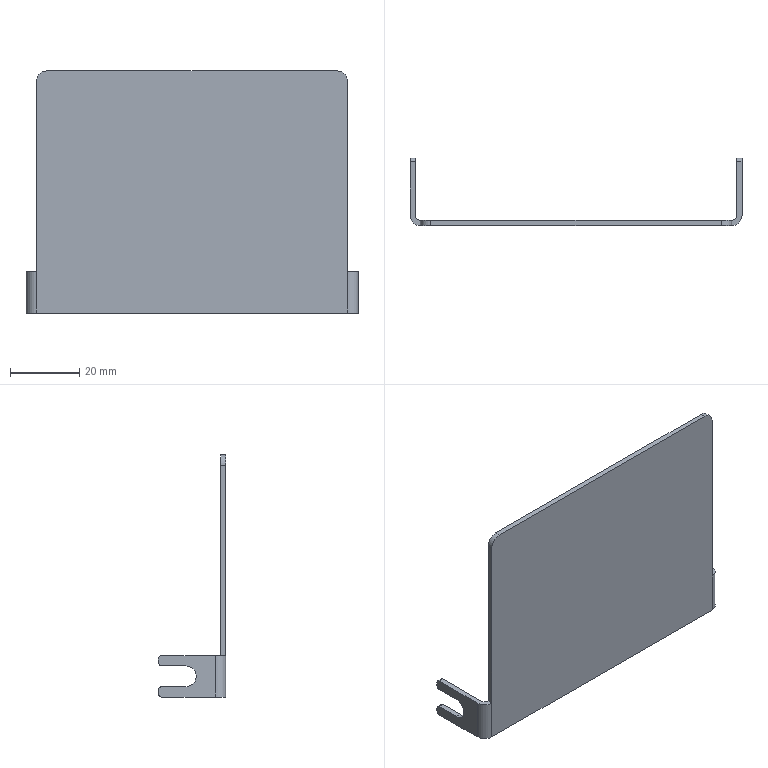Part | NX | features BREP 1 | 1 solid | 36 faces | box 96 x 19.5 x 70 mm | volume 9976 mm3 | plane 20 | cylinder 16 | commonest cylinder face diameters 2 x8 6 x6 3 x2
STEP:
#1=CARTESIAN_POINT('',(-45.,-1.5,67.));
#2=VERTEX_POINT('',#1);
#3=CARTESIAN_POINT('',(-42.,-1.5,70.));
#4=VERTEX_POINT('',#3);
#5=CARTESIAN_POINT('',(-42.,-1.5,67.));
#6=DIRECTION('',(0.,1.,0.));
#7=DIRECTION('',(1.,0.,0.));
#8=AXIS2_PLACEMENT_3D('',#5,#6,#7);
#9=CIRCLE('',#8,3.);
#10=EDGE_CURVE('',#2,#4,#9,.T.);
#11=ORIENTED_EDGE('',*,*,#10,.F.);
#12=CARTESIAN_POINT('',(-45.,-1.5,12.));
#13=VERTEX_POINT('',#12);
#14=CARTESIAN_POINT('',(-45.,-1.5,70.));
#15=DIRECTION('',(0.,0.,1.));
#16=VECTOR('',#15,1000.);
#17=LINE('',#14,#16);
#18=EDGE_CURVE('',#13,#2,#17,.T.);
#19=ORIENTED_EDGE('',*,*,#18,.F.);
#20=CARTESIAN_POINT('',(-45.,-1.5,0.));
#21=VERTEX_POINT('',#20);
#22=CARTESIAN_POINT('',(-45.,-1.5,70.));
#23=DIRECTION('',(0.,0.,1.));
#24=VECTOR('',#23,1000.);
#25=LINE('',#22,#24);
#26=EDGE_CURVE('',#21,#13,#25,.T.);
#27=ORIENTED_EDGE('',*,*,#26,.F.);
#28=CARTESIAN_POINT('',(45.,-1.5,0.));
#29=VERTEX_POINT('',#28);
#30=CARTESIAN_POINT('',(-46.5,-1.5,0.));
#31=DIRECTION('',(-1.,0.,0.));
#32=VECTOR('',#31,1000.);
#33=LINE('',#30,#32);
#34=EDGE_CURVE('',#29,#21,#33,.T.);
#35=ORIENTED_EDGE('',*,*,#34,.F.);
#36=CARTESIAN_POINT('',(45.,-1.5,12.));
#37=VERTEX_POINT('',#36);
#38=CARTESIAN_POINT('',(45.,-1.5,70.));
#39=DIRECTION('',(0.,0.,-1.));
#40=VECTOR('',#39,1000.);
#41=LINE('',#38,#40);
#42=EDGE_CURVE('',#37,#29,#41,.T.);
#43=ORIENTED_EDGE('',*,*,#42,.F.);
#44=CARTESIAN_POINT('',(45.,-1.5,67.));
#45=VERTEX_POINT('',#44);
#46=CARTESIAN_POINT('',(45.,-1.5,70.));
#47=DIRECTION('',(0.,0.,-1.));
#48=VECTOR('',#47,1000.);
#49=LINE('',#46,#48);
#50=EDGE_CURVE('',#45,#37,#49,.T.);
#51=ORIENTED_EDGE('',*,*,#50,.F.);
#52=CARTESIAN_POINT('',(42.,-1.5,70.));
#53=VERTEX_POINT('',#52);
#54=CARTESIAN_POINT('',(42.,-1.5,67.));
#55=DIRECTION('',(0.,1.,0.));
#56=DIRECTION('',(-1.,0.,0.));
#57=AXIS2_PLACEMENT_3D('',#54,#55,#56);
#58=CIRCLE('',#57,3.);
#59=EDGE_CURVE('',#53,#45,#58,.T.);
#60=ORIENTED_EDGE('',*,*,#59,.F.);
#61=CARTESIAN_POINT('',(-46.5,-1.5,70.));
#62=DIRECTION('',(1.,0.,0.));
#63=VECTOR('',#62,1000.);
#64=LINE('',#61,#63);
#65=EDGE_CURVE('',#4,#53,#64,.T.);
#66=ORIENTED_EDGE('',*,*,#65,.F.);
#67=EDGE_LOOP('',(#11,#19,#27,#35,#43,#51,#60,#66));
#68=FACE_BOUND('',#67,.T.);
#69=CARTESIAN_POINT('',(-46.5,-1.5,70.));
#70=DIRECTION('',(0.,1.,0.));
#71=DIRECTION('',(1.,0.,0.));
#72=AXIS2_PLACEMENT_3D('',#69,#70,#71);
#73=PLANE('',#72);
#74=ADVANCED_FACE('',(#68),#73,.F.);
#75=ORIENTED_EDGE('',*,*,#65,.T.);
#76=CARTESIAN_POINT('',(42.,0.,70.));
#77=VERTEX_POINT('',#76);
#78=CARTESIAN_POINT('',(42.,1.5,70.));
#79=DIRECTION('',(0.,1.,0.));
#80=VECTOR('',#79,1000.);
#81=LINE('',#78,#80);
#82=EDGE_CURVE('',#53,#77,#81,.T.);
#83=ORIENTED_EDGE('',*,*,#82,.T.);
#84=CARTESIAN_POINT('',(-42.,0.,70.));
#85=VERTEX_POINT('',#84);
#86=CARTESIAN_POINT('',(-48.,0.,70.));
#87=DIRECTION('',(-1.,0.,0.));
#88=VECTOR('',#87,1000.);
#89=LINE('',#86,#88);
#90=EDGE_CURVE('',#77,#85,#89,.T.);
#91=ORIENTED_EDGE('',*,*,#90,.T.);
#92=CARTESIAN_POINT('',(-42.,1.5,70.));
#93=DIRECTION('',(0.,-1.,0.));
#94=VECTOR('',#93,1000.);
#95=LINE('',#92,#94);
#96=EDGE_CURVE('',#85,#4,#95,.T.);
#97=ORIENTED_EDGE('',*,*,#96,.T.);
#98=EDGE_LOOP('',(#75,#83,#91,#97));
#99=FACE_BOUND('',#98,.T.);
#100=CARTESIAN_POINT('',(-48.,1.5,70.));
#101=DIRECTION('',(0.,0.,1.));
#102=DIRECTION('',(-1.,0.,0.));
#103=AXIS2_PLACEMENT_3D('',#100,#101,#102);
#104=PLANE('',#103);
#105=ADVANCED_FACE('',(#99),#104,.T.);
#106=ORIENTED_EDGE('',*,*,#10,.T.);
#107=ORIENTED_EDGE('',*,*,#96,.F.);
#108=CARTESIAN_POINT('',(-45.,0.,67.));
#109=VERTEX_POINT('',#108);
#110=CARTESIAN_POINT('',(-42.,0.,67.));
#111=DIRECTION('',(0.,-1.,0.));
#112=DIRECTION('',(1.,0.,0.));
#113=AXIS2_PLACEMENT_3D('',#110,#111,#112);
#114=CIRCLE('',#113,3.);
#115=EDGE_CURVE('',#85,#109,#114,.T.);
#116=ORIENTED_EDGE('',*,*,#115,.T.);
#117=CARTESIAN_POINT('',(-45.,1.5,67.));
#118=DIRECTION('',(0.,-1.,0.));
#119=VECTOR('',#118,1000.);
#120=LINE('',#117,#119);
#121=EDGE_CURVE('',#109,#2,#120,.T.);
#122=ORIENTED_EDGE('',*,*,#121,.T.);
#123=EDGE_LOOP('',(#106,#107,#116,#122));
#124=FACE_BOUND('',#123,.T.);
#125=CARTESIAN_POINT('',(-42.,1.5,67.));
#126=DIRECTION('',(0.,-1.,0.));
#127=DIRECTION('',(-1.,0.,0.));
#128=AXIS2_PLACEMENT_3D('',#125,#126,#127);
#129=CYLINDRICAL_SURFACE('',#128,3.);
#130=ADVANCED_FACE('',(#124),#129,.T.);
#131=CARTESIAN_POINT('',(-45.,0.,12.));
#132=VERTEX_POINT('',#131);
#133=CARTESIAN_POINT('',(-45.,0.,0.));
#134=DIRECTION('',(0.,0.,-1.));
#135=VECTOR('',#134,1000.);
#136=LINE('',#133,#135);
#137=EDGE_CURVE('',#109,#132,#136,.T.);
#138=ORIENTED_EDGE('',*,*,#137,.T.);
#139=CARTESIAN_POINT('',(-45.,-1.5,12.));
#140=DIRECTION('',(0.,1.,0.));
#141=VECTOR('',#140,1000.);
#142=LINE('',#139,#141);
#143=EDGE_CURVE('',#13,#132,#142,.T.);
#144=ORIENTED_EDGE('',*,*,#143,.F.);
#145=ORIENTED_EDGE('',*,*,#18,.T.);
#146=ORIENTED_EDGE('',*,*,#121,.F.);
#147=EDGE_LOOP('',(#138,#144,#145,#146));
#148=FACE_BOUND('',#147,.T.);
#149=CARTESIAN_POINT('',(-45.,0.,0.));
#150=DIRECTION('',(-1.,0.,0.));
#151=DIRECTION('',(0.,1.,0.));
#152=AXIS2_PLACEMENT_3D('',#149,#150,#151);
#153=PLANE('',#152);
#154=ADVANCED_FACE('',(#148),#153,.T.);
#155=CARTESIAN_POINT('',(-48.,1.5,0.));
#156=VERTEX_POINT('',#155);
#157=CARTESIAN_POINT('',(-45.,1.5,0.));
#158=DIRECTION('',(0.,0.,1.));
#159=DIRECTION('',(-1.,0.,0.));
#160=AXIS2_PLACEMENT_3D('',#157,#158,#159);
#161=CIRCLE('',#160,3.);
#162=EDGE_CURVE('',#156,#21,#161,.T.);
#163=ORIENTED_EDGE('',*,*,#162,.T.);
#164=ORIENTED_EDGE('',*,*,#26,.T.);
#165=CARTESIAN_POINT('',(-48.,1.5,12.));
#166=VERTEX_POINT('',#165);
#167=CARTESIAN_POINT('',(-45.,1.5,12.));
#168=DIRECTION('',(0.,0.,-1.));
#169=DIRECTION('',(-1.,0.,0.));
#170=AXIS2_PLACEMENT_3D('',#167,#168,#169);
#171=CIRCLE('',#170,3.);
#172=EDGE_CURVE('',#13,#166,#171,.T.);
#173=ORIENTED_EDGE('',*,*,#172,.T.);
#174=CARTESIAN_POINT('',(-48.,1.5,70.));
#175=DIRECTION('',(0.,0.,-1.));
#176=VECTOR('',#175,1000.);
#177=LINE('',#174,#176);
#178=EDGE_CURVE('',#166,#156,#177,.T.);
#179=ORIENTED_EDGE('',*,*,#178,.T.);
#180=EDGE_LOOP('',(#163,#164,#173,#179));
#181=FACE_BOUND('',#180,.T.);
#182=CARTESIAN_POINT('',(-45.,1.5,70.));
#183=DIRECTION('',(0.,0.,-1.));
#184=DIRECTION('',(1.,0.,0.));
#185=AXIS2_PLACEMENT_3D('',#182,#183,#184);
#186=CYLINDRICAL_SURFACE('',#185,3.);
#187=ADVANCED_FACE('',(#181),#186,.T.);
#188=ORIENTED_EDGE('',*,*,#34,.T.);
#189=ORIENTED_EDGE('',*,*,#162,.F.);
#190=CARTESIAN_POINT('',(-48.,17.,0.));
#191=VERTEX_POINT('',#190);
#192=CARTESIAN_POINT('',(-48.,18.,0.));
#193=DIRECTION('',(0.,1.,0.));
#194=VECTOR('',#193,1000.);
#195=LINE('',#192,#194);
#196=EDGE_CURVE('',#156,#191,#195,.T.);
#197=ORIENTED_EDGE('',*,*,#196,.T.);
#198=CARTESIAN_POINT('',(-46.5,17.,0.));
#199=VERTEX_POINT('',#198);
#200=CARTESIAN_POINT('',(-45.,17.,0.));
#201=DIRECTION('',(-1.,0.,0.));
#202=VECTOR('',#201,1000.);
#203=LINE('',#200,#202);
#204=EDGE_CURVE('',#199,#191,#203,.T.);
#205=ORIENTED_EDGE('',*,*,#204,.F.);
#206=CARTESIAN_POINT('',(-46.5,1.5,0.));
#207=VERTEX_POINT('',#206);
#208=CARTESIAN_POINT('',(-46.5,-1.5,0.));
#209=DIRECTION('',(0.,-1.,0.));
#210=VECTOR('',#209,1000.);
#211=LINE('',#208,#210);
#212=EDGE_CURVE('',#199,#207,#211,.T.);
#213=ORIENTED_EDGE('',*,*,#212,.T.);
#214=CARTESIAN_POINT('',(-45.,0.,0.));
#215=VERTEX_POINT('',#214);
#216=CARTESIAN_POINT('',(-45.,1.5,0.));
#217=DIRECTION('',(0.,0.,1.));
#218=DIRECTION('',(-1.,0.,0.));
#219=AXIS2_PLACEMENT_3D('',#216,#217,#218);
#220=CIRCLE('',#219,1.5);
#221=EDGE_CURVE('',#207,#215,#220,.T.);
#222=ORIENTED_EDGE('',*,*,#221,.T.);
#223=CARTESIAN_POINT('',(45.,0.,0.));
#224=VERTEX_POINT('',#223);
#225=CARTESIAN_POINT('',(48.,0.,0.));
#226=DIRECTION('',(1.,0.,0.));
#227=VECTOR('',#226,1000.);
#228=LINE('',#225,#227);
#229=EDGE_CURVE('',#215,#224,#228,.T.);
#230=ORIENTED_EDGE('',*,*,#229,.T.);
#231=CARTESIAN_POINT('',(46.5,1.5,0.));
#232=VERTEX_POINT('',#231);
#233=CARTESIAN_POINT('',(45.,1.5,0.));
#234=DIRECTION('',(0.,0.,1.));
#235=DIRECTION('',(-1.,0.,0.));
#236=AXIS2_PLACEMENT_3D('',#233,#234,#235);
#237=CIRCLE('',#236,1.5);
#238=EDGE_CURVE('',#224,#232,#237,.T.);
#239=ORIENTED_EDGE('',*,*,#238,.T.);
#240=CARTESIAN_POINT('',(46.5,17.,0.));
#241=VERTEX_POINT('',#240);
#242=CARTESIAN_POINT('',(46.5,0.,0.));
#243=DIRECTION('',(0.,-1.,0.));
#244=VECTOR('',#243,1000.);
#245=LINE('',#242,#244);
#246=EDGE_CURVE('',#241,#232,#245,.T.);
#247=ORIENTED_EDGE('',*,*,#246,.F.);
#248=CARTESIAN_POINT('',(48.,17.,0.));
#249=VERTEX_POINT('',#248);
#250=CARTESIAN_POINT('',(45.,17.,0.));
#251=DIRECTION('',(1.,0.,0.));
#252=VECTOR('',#251,1000.);
#253=LINE('',#250,#252);
#254=EDGE_CURVE('',#241,#249,#253,.T.);
#255=ORIENTED_EDGE('',*,*,#254,.T.);
#256=CARTESIAN_POINT('',(48.,1.5,0.));
#257=VERTEX_POINT('',#256);
#258=CARTESIAN_POINT('',(48.,0.,0.));
#259=DIRECTION('',(0.,-1.,0.));
#260=VECTOR('',#259,1000.);
#261=LINE('',#258,#260);
#262=EDGE_CURVE('',#249,#257,#261,.T.);
#263=ORIENTED_EDGE('',*,*,#262,.T.);
#264=CARTESIAN_POINT('',(45.,1.5,0.));
#265=DIRECTION('',(0.,0.,1.));
#266=DIRECTION('',(-1.,0.,0.));
#267=AXIS2_PLACEMENT_3D('',#264,#265,#266);
#268=CIRCLE('',#267,3.);
#269=EDGE_CURVE('',#29,#257,#268,.T.);
#270=ORIENTED_EDGE('',*,*,#269,.F.);
#271=EDGE_LOOP('',(#188,#189,#197,#205,#213,#222,#230,#239,#247,#255,#263,#270));
#272=FACE_BOUND('',#271,.T.);
#273=CARTESIAN_POINT('',(48.,1.5,0.));
#274=DIRECTION('',(0.,0.,-1.));
#275=DIRECTION('',(1.,0.,0.));
#276=AXIS2_PLACEMENT_3D('',#273,#274,#275);
#277=PLANE('',#276);
#278=ADVANCED_FACE('',(#272),#277,.T.);
#279=ORIENTED_EDGE('',*,*,#42,.T.);
#280=ORIENTED_EDGE('',*,*,#269,.T.);
#281=CARTESIAN_POINT('',(48.,1.5,12.));
#282=VERTEX_POINT('',#281);
#283=CARTESIAN_POINT('',(48.,1.5,70.));
#284=DIRECTION('',(0.,0.,1.));
#285=VECTOR('',#284,1000.);
#286=LINE('',#283,#285);
#287=EDGE_CURVE('',#257,#282,#286,.T.);
#288=ORIENTED_EDGE('',*,*,#287,.T.);
#289=CARTESIAN_POINT('',(45.,1.5,12.));
#290=DIRECTION('',(0.,0.,-1.));
#291=DIRECTION('',(-1.,0.,0.));
#292=AXIS2_PLACEMENT_3D('',#289,#290,#291);
#293=CIRCLE('',#292,3.);
#294=EDGE_CURVE('',#282,#37,#293,.T.);
#295=ORIENTED_EDGE('',*,*,#294,.T.);
#296=EDGE_LOOP('',(#279,#280,#288,#295));
#297=FACE_BOUND('',#296,.T.);
#298=CARTESIAN_POINT('',(45.,1.5,70.));
#299=DIRECTION('',(0.,0.,-1.));
#300=DIRECTION('',(1.,0.,0.));
#301=AXIS2_PLACEMENT_3D('',#298,#299,#300);
#302=CYLINDRICAL_SURFACE('',#301,3.);
#303=ADVANCED_FACE('',(#297),#302,.T.);
#304=ORIENTED_EDGE('',*,*,#50,.T.);
#305=CARTESIAN_POINT('',(45.,0.,12.));
#306=VERTEX_POINT('',#305);
#307=CARTESIAN_POINT('',(45.,0.,12.));
#308=DIRECTION('',(0.,1.,0.));
#309=VECTOR('',#308,1000.);
#310=LINE('',#307,#309);
#311=EDGE_CURVE('',#37,#306,#310,.T.);
#312=ORIENTED_EDGE('',*,*,#311,.T.);
#313=CARTESIAN_POINT('',(45.,0.,67.));
#314=VERTEX_POINT('',#313);
#315=CARTESIAN_POINT('',(45.,0.,0.));
#316=DIRECTION('',(0.,0.,1.));
#317=VECTOR('',#316,1000.);
#318=LINE('',#315,#317);
#319=EDGE_CURVE('',#306,#314,#318,.T.);
#320=ORIENTED_EDGE('',*,*,#319,.T.);
#321=CARTESIAN_POINT('',(45.,0.,67.));
#322=DIRECTION('',(0.,-1.,0.));
#323=VECTOR('',#322,1000.);
#324=LINE('',#321,#323);
#325=EDGE_CURVE('',#314,#45,#324,.T.);
#326=ORIENTED_EDGE('',*,*,#325,.T.);
#327=EDGE_LOOP('',(#304,#312,#320,#326));
#328=FACE_BOUND('',#327,.T.);
#329=CARTESIAN_POINT('',(45.,0.,0.));
#330=DIRECTION('',(1.,0.,0.));
#331=DIRECTION('',(0.,-1.,0.));
#332=AXIS2_PLACEMENT_3D('',#329,#330,#331);
#333=PLANE('',#332);
#334=ADVANCED_FACE('',(#328),#333,.T.);
#335=CARTESIAN_POINT('',(42.,0.,67.));
#336=DIRECTION('',(0.,-1.,0.));
#337=DIRECTION('',(-1.,0.,0.));
#338=AXIS2_PLACEMENT_3D('',#335,#336,#337);
#339=CIRCLE('',#338,3.);
#340=EDGE_CURVE('',#314,#77,#339,.T.);
#341=ORIENTED_EDGE('',*,*,#340,.T.);
#342=ORIENTED_EDGE('',*,*,#82,.F.);
#343=ORIENTED_EDGE('',*,*,#59,.T.);
#344=ORIENTED_EDGE('',*,*,#325,.F.);
#345=EDGE_LOOP('',(#341,#342,#343,#344));
#346=FACE_BOUND('',#345,.T.);
#347=CARTESIAN_POINT('',(42.,1.5,67.));
#348=DIRECTION('',(0.,1.,0.));
#349=DIRECTION('',(1.,0.,0.));
#350=AXIS2_PLACEMENT_3D('',#347,#348,#349);
#351=CYLINDRICAL_SURFACE('',#350,3.);
#352=ADVANCED_FACE('',(#346),#351,.T.);
#353=ORIENTED_EDGE('',*,*,#229,.F.);
#354=CARTESIAN_POINT('',(-45.,0.,70.));
#355=DIRECTION('',(0.,0.,1.));
#356=VECTOR('',#355,1000.);
#357=LINE('',#354,#356);
#358=EDGE_CURVE('',#215,#132,#357,.T.);
#359=ORIENTED_EDGE('',*,*,#358,.T.);
#360=ORIENTED_EDGE('',*,*,#137,.F.);
#361=ORIENTED_EDGE('',*,*,#115,.F.);
#362=ORIENTED_EDGE('',*,*,#90,.F.);
#363=ORIENTED_EDGE('',*,*,#340,.F.);
#364=ORIENTED_EDGE('',*,*,#319,.F.);
#365=CARTESIAN_POINT('',(45.,0.,70.));
#366=DIRECTION('',(0.,0.,-1.));
#367=VECTOR('',#366,1000.);
#368=LINE('',#365,#367);
#369=EDGE_CURVE('',#306,#224,#368,.T.);
#370=ORIENTED_EDGE('',*,*,#369,.T.);
#371=EDGE_LOOP('',(#353,#359,#360,#361,#362,#363,#364,#370));
#372=FACE_BOUND('',#371,.T.);
#373=CARTESIAN_POINT('',(-46.5,0.,70.));
#374=DIRECTION('',(0.,1.,0.));
#375=DIRECTION('',(1.,0.,0.));
#376=AXIS2_PLACEMENT_3D('',#373,#374,#375);
#377=PLANE('',#376);
#378=ADVANCED_FACE('',(#372),#377,.T.);
#379=CARTESIAN_POINT('',(-48.,18.,1.));
#380=VERTEX_POINT('',#379);
#381=CARTESIAN_POINT('',(-48.,17.,1.));
#382=DIRECTION('',(1.,0.,0.));
#383=DIRECTION('',(0.,0.,-1.));
#384=AXIS2_PLACEMENT_3D('',#381,#382,#383);
#385=CIRCLE('',#384,1.);
#386=EDGE_CURVE('',#191,#380,#385,.T.);
#387=ORIENTED_EDGE('',*,*,#386,.F.);
#388=ORIENTED_EDGE('',*,*,#196,.F.);
#389=ORIENTED_EDGE('',*,*,#178,.F.);
#390=CARTESIAN_POINT('',(-48.,17.,12.));
#391=VERTEX_POINT('',#390);
#392=CARTESIAN_POINT('',(-48.,18.,12.));
#393=DIRECTION('',(0.,-1.,0.));
#394=VECTOR('',#393,1000.);
#395=LINE('',#392,#394);
#396=EDGE_CURVE('',#391,#166,#395,.T.);
#397=ORIENTED_EDGE('',*,*,#396,.F.);
#398=CARTESIAN_POINT('',(-48.,18.,11.));
#399=VERTEX_POINT('',#398);
#400=CARTESIAN_POINT('',(-48.,17.,11.));
#401=DIRECTION('',(1.,0.,0.));
#402=DIRECTION('',(0.,0.,1.));
#403=AXIS2_PLACEMENT_3D('',#400,#401,#402);
#404=CIRCLE('',#403,1.);
#405=EDGE_CURVE('',#399,#391,#404,.T.);
#406=ORIENTED_EDGE('',*,*,#405,.F.);
#407=CARTESIAN_POINT('',(-48.,18.,10.));
#408=VERTEX_POINT('',#407);
#409=CARTESIAN_POINT('',(-48.,18.,70.));
#410=DIRECTION('',(0.,0.,1.));
#411=VECTOR('',#410,1000.);
#412=LINE('',#409,#411);
#413=EDGE_CURVE('',#408,#399,#412,.T.);
#414=ORIENTED_EDGE('',*,*,#413,.F.);
#415=CARTESIAN_POINT('',(-48.,17.,9.));
#416=VERTEX_POINT('',#415);
#417=CARTESIAN_POINT('',(-48.,17.,10.));
#418=DIRECTION('',(1.,0.,0.));
#419=DIRECTION('',(0.,0.,1.));
#420=AXIS2_PLACEMENT_3D('',#417,#418,#419);
#421=CIRCLE('',#420,1.);
#422=EDGE_CURVE('',#416,#408,#421,.T.);
#423=ORIENTED_EDGE('',*,*,#422,.F.);
#424=CARTESIAN_POINT('',(-48.,10.,9.));
#425=VERTEX_POINT('',#424);
#426=CARTESIAN_POINT('',(-48.,18.,9.));
#427=DIRECTION('',(0.,1.,0.));
#428=VECTOR('',#427,1000.);
#429=LINE('',#426,#428);
#430=EDGE_CURVE('',#425,#416,#429,.T.);
#431=ORIENTED_EDGE('',*,*,#430,.F.);
#432=CARTESIAN_POINT('',(-48.,10.,3.));
#433=VERTEX_POINT('',#432);
#434=CARTESIAN_POINT('',(-48.,10.,6.));
#435=DIRECTION('',(-1.,0.,0.));
#436=DIRECTION('',(0.,1.,0.));
#437=AXIS2_PLACEMENT_3D('',#434,#435,#436);
#438=CIRCLE('',#437,3.);
#439=EDGE_CURVE('',#433,#425,#438,.T.);
#440=ORIENTED_EDGE('',*,*,#439,.F.);
#441=CARTESIAN_POINT('',(-48.,17.,3.));
#442=VERTEX_POINT('',#441);
#443=CARTESIAN_POINT('',(-48.,18.,3.));
#444=DIRECTION('',(0.,-1.,0.));
#445=VECTOR('',#444,1000.);
#446=LINE('',#443,#445);
#447=EDGE_CURVE('',#442,#433,#446,.T.);
#448=ORIENTED_EDGE('',*,*,#447,.F.);
#449=CARTESIAN_POINT('',(-48.,18.,2.));
#450=VERTEX_POINT('',#449);
#451=CARTESIAN_POINT('',(-48.,17.,2.));
#452=DIRECTION('',(1.,0.,0.));
#453=DIRECTION('',(0.,0.,1.));
#454=AXIS2_PLACEMENT_3D('',#451,#452,#453);
#455=CIRCLE('',#454,1.);
#456=EDGE_CURVE('',#450,#442,#455,.T.);
#457=ORIENTED_EDGE('',*,*,#456,.F.);
#458=CARTESIAN_POINT('',(-48.,18.,70.));
#459=DIRECTION('',(0.,0.,1.));
#460=VECTOR('',#459,1000.);
#461=LINE('',#458,#460);
#462=EDGE_CURVE('',#380,#450,#461,.T.);
#463=ORIENTED_EDGE('',*,*,#462,.F.);
#464=EDGE_LOOP('',(#387,#388,#389,#397,#406,#414,#423,#431,#440,#448,#457,#463));
#465=FACE_BOUND('',#464,.T.);
#466=CARTESIAN_POINT('',(-48.,18.,70.));
#467=DIRECTION('',(1.,0.,0.));
#468=DIRECTION('',(0.,-1.,0.));
#469=AXIS2_PLACEMENT_3D('',#466,#467,#468);
#470=PLANE('',#469);
#471=ADVANCED_FACE('',(#465),#470,.F.);
#472=ORIENTED_EDGE('',*,*,#143,.T.);
#473=CARTESIAN_POINT('',(-46.5,1.5,12.));
#474=VERTEX_POINT('',#473);
#475=CARTESIAN_POINT('',(-45.,1.5,12.));
#476=DIRECTION('',(0.,0.,-1.));
#477=DIRECTION('',(-1.,0.,0.));
#478=AXIS2_PLACEMENT_3D('',#475,#476,#477);
#479=CIRCLE('',#478,1.5);
#480=EDGE_CURVE('',#132,#474,#479,.T.);
#481=ORIENTED_EDGE('',*,*,#480,.T.);
#482=CARTESIAN_POINT('',(-46.5,17.,12.));
#483=VERTEX_POINT('',#482);
#484=CARTESIAN_POINT('',(-46.5,-1.5,12.));
#485=DIRECTION('',(0.,1.,0.));
#486=VECTOR('',#485,1000.);
#487=LINE('',#484,#486);
#488=EDGE_CURVE('',#474,#483,#487,.T.);
#489=ORIENTED_EDGE('',*,*,#488,.T.);
#490=CARTESIAN_POINT('',(-45.,17.,12.));
#491=DIRECTION('',(-1.,0.,0.));
#492=VECTOR('',#491,1000.);
#493=LINE('',#490,#492);
#494=EDGE_CURVE('',#483,#391,#493,.T.);
#495=ORIENTED_EDGE('',*,*,#494,.T.);
#496=ORIENTED_EDGE('',*,*,#396,.T.);
#497=ORIENTED_EDGE('',*,*,#172,.F.);
#498=EDGE_LOOP('',(#472,#481,#489,#495,#496,#497));
#499=FACE_BOUND('',#498,.T.);
#500=CARTESIAN_POINT('',(-45.,-1.5,12.));
#501=DIRECTION('',(0.,0.,1.));
#502=DIRECTION('',(-1.,0.,0.));
#503=AXIS2_PLACEMENT_3D('',#500,#501,#502);
#504=PLANE('',#503);
#505=ADVANCED_FACE('',(#499),#504,.T.);
#506=CARTESIAN_POINT('',(46.5,17.,12.));
#507=VERTEX_POINT('',#506);
#508=CARTESIAN_POINT('',(48.,17.,12.));
#509=VERTEX_POINT('',#508);
#510=CARTESIAN_POINT('',(45.,17.,12.));
#511=DIRECTION('',(1.,0.,0.));
#512=VECTOR('',#511,1000.);
#513=LINE('',#510,#512);
#514=EDGE_CURVE('',#507,#509,#513,.T.);
#515=ORIENTED_EDGE('',*,*,#514,.F.);
#516=CARTESIAN_POINT('',(46.5,1.5,12.));
#517=VERTEX_POINT('',#516);
#518=CARTESIAN_POINT('',(46.5,-1.5,12.));
#519=DIRECTION('',(0.,1.,0.));
#520=VECTOR('',#519,1000.);
#521=LINE('',#518,#520);
#522=EDGE_CURVE('',#517,#507,#521,.T.);
#523=ORIENTED_EDGE('',*,*,#522,.F.);
#524=CARTESIAN_POINT('',(45.,1.5,12.));
#525=DIRECTION('',(0.,0.,1.));
#526=DIRECTION('',(-1.,0.,0.));
#527=AXIS2_PLACEMENT_3D('',#524,#525,#526);
#528=CIRCLE('',#527,1.5);
#529=EDGE_CURVE('',#306,#517,#528,.T.);
#530=ORIENTED_EDGE('',*,*,#529,.F.);
#531=ORIENTED_EDGE('',*,*,#311,.F.);
#532=ORIENTED_EDGE('',*,*,#294,.F.);
#533=CARTESIAN_POINT('',(48.,-1.5,12.));
#534=DIRECTION('',(0.,-1.,0.));
#535=VECTOR('',#534,1000.);
#536=LINE('',#533,#535);
#537=EDGE_CURVE('',#509,#282,#536,.T.);
#538=ORIENTED_EDGE('',*,*,#537,.F.);
#539=EDGE_LOOP('',(#515,#523,#530,#531,#532,#538));
#540=FACE_BOUND('',#539,.T.);
#541=CARTESIAN_POINT('',(45.,-1.5,12.));
#542=DIRECTION('',(0.,0.,-1.));
#543=DIRECTION('',(1.,0.,0.));
#544=AXIS2_PLACEMENT_3D('',#541,#542,#543);
#545=PLANE('',#544);
#546=ADVANCED_FACE('',(#540),#545,.F.);
#547=CARTESIAN_POINT('',(48.,18.,11.));
#548=VERTEX_POINT('',#547);
#549=CARTESIAN_POINT('',(48.,17.,11.));
#550=DIRECTION('',(-1.,0.,0.));
#551=DIRECTION('',(0.,0.,1.));
#552=AXIS2_PLACEMENT_3D('',#549,#550,#551);
#553=CIRCLE('',#552,1.);
#554=EDGE_CURVE('',#509,#548,#553,.T.);
#555=ORIENTED_EDGE('',*,*,#554,.F.);
#556=ORIENTED_EDGE('',*,*,#537,.T.);
#557=ORIENTED_EDGE('',*,*,#287,.F.);
#558=ORIENTED_EDGE('',*,*,#262,.F.);
#559=CARTESIAN_POINT('',(48.,18.,1.));
#560=VERTEX_POINT('',#559);
#561=CARTESIAN_POINT('',(48.,17.,1.));
#562=DIRECTION('',(-1.,0.,0.));
#563=DIRECTION('',(0.,0.,-1.));
#564=AXIS2_PLACEMENT_3D('',#561,#562,#563);
#565=CIRCLE('',#564,1.);
#566=EDGE_CURVE('',#560,#249,#565,.T.);
#567=ORIENTED_EDGE('',*,*,#566,.F.);
#568=CARTESIAN_POINT('',(48.,18.,2.));
#569=VERTEX_POINT('',#568);
#570=CARTESIAN_POINT('',(48.,18.,70.));
#571=DIRECTION('',(0.,0.,-1.));
#572=VECTOR('',#571,1000.);
#573=LINE('',#570,#572);
#574=EDGE_CURVE('',#569,#560,#573,.T.);
#575=ORIENTED_EDGE('',*,*,#574,.F.);
#576=CARTESIAN_POINT('',(48.,17.,3.));
#577=VERTEX_POINT('',#576);
#578=CARTESIAN_POINT('',(48.,17.,2.));
#579=DIRECTION('',(-1.,0.,0.));
#580=DIRECTION('',(0.,0.,1.));
#581=AXIS2_PLACEMENT_3D('',#578,#579,#580);
#582=CIRCLE('',#581,1.);
#583=EDGE_CURVE('',#577,#569,#582,.T.);
#584=ORIENTED_EDGE('',*,*,#583,.F.);
#585=CARTESIAN_POINT('',(48.,10.,3.));
#586=VERTEX_POINT('',#585);
#587=CARTESIAN_POINT('',(48.,0.,3.));
#588=DIRECTION('',(0.,1.,0.));
#589=VECTOR('',#588,1000.);
#590=LINE('',#587,#589);
#591=EDGE_CURVE('',#586,#577,#590,.T.);
#592=ORIENTED_EDGE('',*,*,#591,.F.);
#593=CARTESIAN_POINT('',(48.,10.,9.));
#594=VERTEX_POINT('',#593);
#595=CARTESIAN_POINT('',(48.,10.,6.));
#596=DIRECTION('',(1.,0.,0.));
#597=DIRECTION('',(0.,1.,0.));
#598=AXIS2_PLACEMENT_3D('',#595,#596,#597);
#599=CIRCLE('',#598,3.);
#600=EDGE_CURVE('',#594,#586,#599,.T.);
#601=ORIENTED_EDGE('',*,*,#600,.F.);
#602=CARTESIAN_POINT('',(48.,17.,9.));
#603=VERTEX_POINT('',#602);
#604=CARTESIAN_POINT('',(48.,0.,9.));
#605=DIRECTION('',(0.,-1.,0.));
#606=VECTOR('',#605,1000.);
#607=LINE('',#604,#606);
#608=EDGE_CURVE('',#603,#594,#607,.T.);
#609=ORIENTED_EDGE('',*,*,#608,.F.);
#610=CARTESIAN_POINT('',(48.,18.,10.));
#611=VERTEX_POINT('',#610);
#612=CARTESIAN_POINT('',(48.,17.,10.));
#613=DIRECTION('',(-1.,0.,0.));
#614=DIRECTION('',(0.,0.,1.));
#615=AXIS2_PLACEMENT_3D('',#612,#613,#614);
#616=CIRCLE('',#615,1.);
#617=EDGE_CURVE('',#611,#603,#616,.T.);
#618=ORIENTED_EDGE('',*,*,#617,.F.);
#619=CARTESIAN_POINT('',(48.,18.,70.));
#620=DIRECTION('',(0.,0.,-1.));
#621=VECTOR('',#620,1000.);
#622=LINE('',#619,#621);
#623=EDGE_CURVE('',#548,#611,#622,.T.);
#624=ORIENTED_EDGE('',*,*,#623,.F.);
#625=EDGE_LOOP('',(#555,#556,#557,#558,#567,#575,#584,#592,#601,#609,#618,#624));
#626=FACE_BOUND('',#625,.T.);
#627=CARTESIAN_POINT('',(48.,0.,70.));
#628=DIRECTION('',(-1.,0.,0.));
#629=DIRECTION('',(0.,1.,0.));
#630=AXIS2_PLACEMENT_3D('',#627,#628,#629);
#631=PLANE('',#630);
#632=ADVANCED_FACE('',(#626),#631,.F.);
#633=ORIENTED_EDGE('',*,*,#480,.F.);
#634=ORIENTED_EDGE('',*,*,#358,.F.);
#635=ORIENTED_EDGE('',*,*,#221,.F.);
#636=CARTESIAN_POINT('',(-46.5,1.5,70.));
#637=DIRECTION('',(0.,0.,-1.));
#638=VECTOR('',#637,1000.);
#639=LINE('',#636,#638);
#640=EDGE_CURVE('',#474,#207,#639,.T.);
#641=ORIENTED_EDGE('',*,*,#640,.F.);
#642=EDGE_LOOP('',(#633,#634,#635,#641));
#643=FACE_BOUND('',#642,.T.);
#644=CARTESIAN_POINT('',(-45.,1.5,70.));
#645=DIRECTION('',(0.,0.,-1.));
#646=DIRECTION('',(1.,0.,0.));
#647=AXIS2_PLACEMENT_3D('',#644,#645,#646);
#648=CYLINDRICAL_SURFACE('',#647,1.5);
#649=ADVANCED_FACE('',(#643),#648,.F.);
#650=CARTESIAN_POINT('',(46.5,1.5,70.));
#651=DIRECTION('',(0.,0.,1.));
#652=VECTOR('',#651,1000.);
#653=LINE('',#650,#652);
#654=EDGE_CURVE('',#232,#517,#653,.T.);
#655=ORIENTED_EDGE('',*,*,#654,.F.);
#656=ORIENTED_EDGE('',*,*,#238,.F.);
#657=ORIENTED_EDGE('',*,*,#369,.F.);
#658=ORIENTED_EDGE('',*,*,#529,.T.);
#659=EDGE_LOOP('',(#655,#656,#657,#658));
#660=FACE_BOUND('',#659,.T.);
#661=CARTESIAN_POINT('',(45.,1.5,70.));
#662=DIRECTION('',(0.,0.,-1.));
#663=DIRECTION('',(1.,0.,0.));
#664=AXIS2_PLACEMENT_3D('',#661,#662,#663);
#665=CYLINDRICAL_SURFACE('',#664,1.5);
#666=ADVANCED_FACE('',(#660),#665,.F.);
#667=ORIENTED_EDGE('',*,*,#462,.T.);
#668=CARTESIAN_POINT('',(-46.5,18.,2.));
#669=VERTEX_POINT('',#668);
#670=CARTESIAN_POINT('',(-48.,18.,2.));
#671=DIRECTION('',(1.,0.,0.));
#672=VECTOR('',#671,1000.);
#673=LINE('',#670,#672);
#674=EDGE_CURVE('',#450,#669,#673,.T.);
#675=ORIENTED_EDGE('',*,*,#674,.T.);
#676=CARTESIAN_POINT('',(-46.5,18.,1.));
#677=VERTEX_POINT('',#676);
#678=CARTESIAN_POINT('',(-46.5,18.,70.));
#679=DIRECTION('',(0.,0.,-1.));
#680=VECTOR('',#679,1000.);
#681=LINE('',#678,#680);
#682=EDGE_CURVE('',#669,#677,#681,.T.);
#683=ORIENTED_EDGE('',*,*,#682,.T.);
#684=CARTESIAN_POINT('',(-48.,18.,1.));
#685=DIRECTION('',(-1.,0.,0.));
#686=VECTOR('',#685,1000.);
#687=LINE('',#684,#686);
#688=EDGE_CURVE('',#677,#380,#687,.T.);
#689=ORIENTED_EDGE('',*,*,#688,.T.);
#690=EDGE_LOOP('',(#667,#675,#683,#689));
#691=FACE_BOUND('',#690,.T.);
#692=CARTESIAN_POINT('',(-48.,18.,70.));
#693=DIRECTION('',(0.,1.,0.));
#694=DIRECTION('',(0.,0.,-1.));
#695=AXIS2_PLACEMENT_3D('',#692,#693,#694);
#696=PLANE('',#695);
#697=ADVANCED_FACE('',(#691),#696,.T.);
#698=CARTESIAN_POINT('',(-46.5,17.,1.));
#699=DIRECTION('',(-1.,0.,0.));
#700=DIRECTION('',(0.,0.,-1.));
#701=AXIS2_PLACEMENT_3D('',#698,#699,#700);
#702=CIRCLE('',#701,1.);
#703=EDGE_CURVE('',#677,#199,#702,.T.);
#704=ORIENTED_EDGE('',*,*,#703,.T.);
#705=ORIENTED_EDGE('',*,*,#204,.T.);
#706=ORIENTED_EDGE('',*,*,#386,.T.);
#707=ORIENTED_EDGE('',*,*,#688,.F.);
#708=EDGE_LOOP('',(#704,#705,#706,#707));
#709=FACE_BOUND('',#708,.T.);
#710=CARTESIAN_POINT('',(-45.,17.,1.));
#711=DIRECTION('',(1.,0.,0.));
#712=DIRECTION('',(0.,0.,1.));
#713=AXIS2_PLACEMENT_3D('',#710,#711,#712);
#714=CYLINDRICAL_SURFACE('',#713,1.);
#715=ADVANCED_FACE('',(#709),#714,.T.);
#716=ORIENTED_EDGE('',*,*,#405,.T.);
#717=ORIENTED_EDGE('',*,*,#494,.F.);
#718=CARTESIAN_POINT('',(-46.5,18.,11.));
#719=VERTEX_POINT('',#718);
#720=CARTESIAN_POINT('',(-46.5,17.,11.));
#721=DIRECTION('',(-1.,0.,0.));
#722=DIRECTION('',(0.,0.,1.));
#723=AXIS2_PLACEMENT_3D('',#720,#721,#722);
#724=CIRCLE('',#723,1.);
#725=EDGE_CURVE('',#483,#719,#724,.T.);
#726=ORIENTED_EDGE('',*,*,#725,.T.);
#727=CARTESIAN_POINT('',(-45.,18.,11.));
#728=DIRECTION('',(-1.,0.,0.));
#729=VECTOR('',#728,1000.);
#730=LINE('',#727,#729);
#731=EDGE_CURVE('',#719,#399,#730,.T.);
#732=ORIENTED_EDGE('',*,*,#731,.T.);
#733=EDGE_LOOP('',(#716,#717,#726,#732));
#734=FACE_BOUND('',#733,.T.);
#735=CARTESIAN_POINT('',(-45.,17.,11.));
#736=DIRECTION('',(-1.,0.,0.));
#737=DIRECTION('',(0.,0.,-1.));
#738=AXIS2_PLACEMENT_3D('',#735,#736,#737);
#739=CYLINDRICAL_SURFACE('',#738,1.);
#740=ADVANCED_FACE('',(#734),#739,.T.);
#741=CARTESIAN_POINT('',(-46.5,18.,10.));
#742=VERTEX_POINT('',#741);
#743=CARTESIAN_POINT('',(-46.5,18.,70.));
#744=DIRECTION('',(0.,0.,-1.));
#745=VECTOR('',#744,1000.);
#746=LINE('',#743,#745);
#747=EDGE_CURVE('',#719,#742,#746,.T.);
#748=ORIENTED_EDGE('',*,*,#747,.T.);
#749=CARTESIAN_POINT('',(-48.,18.,10.));
#750=DIRECTION('',(-1.,0.,0.));
#751=VECTOR('',#750,1000.);
#752=LINE('',#749,#751);
#753=EDGE_CURVE('',#742,#408,#752,.T.);
#754=ORIENTED_EDGE('',*,*,#753,.T.);
#755=ORIENTED_EDGE('',*,*,#413,.T.);
#756=ORIENTED_EDGE('',*,*,#731,.F.);
#757=EDGE_LOOP('',(#748,#754,#755,#756));
#758=FACE_BOUND('',#757,.T.);
#759=CARTESIAN_POINT('',(-48.,18.,70.));
#760=DIRECTION('',(0.,1.,0.));
#761=DIRECTION('',(0.,0.,-1.));
#762=AXIS2_PLACEMENT_3D('',#759,#760,#761);
#763=PLANE('',#762);
#764=ADVANCED_FACE('',(#758),#763,.T.);
#765=CARTESIAN_POINT('',(-46.5,17.,9.));
#766=VERTEX_POINT('',#765);
#767=CARTESIAN_POINT('',(-46.5,17.,10.));
#768=DIRECTION('',(-1.,0.,0.));
#769=DIRECTION('',(0.,0.,1.));
#770=AXIS2_PLACEMENT_3D('',#767,#768,#769);
#771=CIRCLE('',#770,1.);
#772=EDGE_CURVE('',#742,#766,#771,.T.);
#773=ORIENTED_EDGE('',*,*,#772,.T.);
#774=CARTESIAN_POINT('',(-48.,17.,9.));
#775=DIRECTION('',(-1.,0.,0.));
#776=VECTOR('',#775,1000.);
#777=LINE('',#774,#776);
#778=EDGE_CURVE('',#766,#416,#777,.T.);
#779=ORIENTED_EDGE('',*,*,#778,.T.);
#780=ORIENTED_EDGE('',*,*,#422,.T.);
#781=ORIENTED_EDGE('',*,*,#753,.F.);
#782=EDGE_LOOP('',(#773,#779,#780,#781));
#783=FACE_BOUND('',#782,.T.);
#784=CARTESIAN_POINT('',(-48.,17.,10.));
#785=DIRECTION('',(-1.,0.,0.));
#786=DIRECTION('',(0.,0.,-1.));
#787=AXIS2_PLACEMENT_3D('',#784,#785,#786);
#788=CYLINDRICAL_SURFACE('',#787,1.);
#789=ADVANCED_FACE('',(#783),#788,.T.);
#790=ORIENTED_EDGE('',*,*,#778,.F.);
#791=CARTESIAN_POINT('',(-46.5,10.,9.));
#792=VERTEX_POINT('',#791);
#793=CARTESIAN_POINT('',(-46.5,18.,9.));
#794=DIRECTION('',(0.,1.,0.));
#795=VECTOR('',#794,1000.);
#796=LINE('',#793,#795);
#797=EDGE_CURVE('',#792,#766,#796,.T.);
#798=ORIENTED_EDGE('',*,*,#797,.F.);
#799=CARTESIAN_POINT('',(-48.,10.,9.));
#800=DIRECTION('',(1.,0.,0.));
#801=VECTOR('',#800,1000.);
#802=LINE('',#799,#801);
#803=EDGE_CURVE('',#425,#792,#802,.T.);
#804=ORIENTED_EDGE('',*,*,#803,.F.);
#805=ORIENTED_EDGE('',*,*,#430,.T.);
#806=EDGE_LOOP('',(#790,#798,#804,#805));
#807=FACE_BOUND('',#806,.T.);
#808=CARTESIAN_POINT('',(-48.,18.,9.));
#809=DIRECTION('',(0.,0.,1.));
#810=DIRECTION('',(-1.,0.,0.));
#811=AXIS2_PLACEMENT_3D('',#808,#809,#810);
#812=PLANE('',#811);
#813=ADVANCED_FACE('',(#807),#812,.F.);
#814=CARTESIAN_POINT('',(-46.5,10.,3.));
#815=VERTEX_POINT('',#814);
#816=CARTESIAN_POINT('',(-48.,10.,3.));
#817=DIRECTION('',(1.,0.,0.));
#818=VECTOR('',#817,1000.);
#819=LINE('',#816,#818);
#820=EDGE_CURVE('',#433,#815,#819,.T.);
#821=ORIENTED_EDGE('',*,*,#820,.F.);
#822=ORIENTED_EDGE('',*,*,#439,.T.);
#823=ORIENTED_EDGE('',*,*,#803,.T.);
#824=CARTESIAN_POINT('',(-46.5,10.,6.));
#825=DIRECTION('',(-1.,0.,0.));
#826=DIRECTION('',(0.,1.,0.));
#827=AXIS2_PLACEMENT_3D('',#824,#825,#826);
#828=CIRCLE('',#827,3.);
#829=EDGE_CURVE('',#815,#792,#828,.T.);
#830=ORIENTED_EDGE('',*,*,#829,.F.);
#831=EDGE_LOOP('',(#821,#822,#823,#830));
#832=FACE_BOUND('',#831,.T.);
#833=CARTESIAN_POINT('',(-48.,10.,6.));
#834=DIRECTION('',(1.,0.,0.));
#835=DIRECTION('',(0.,-1.,0.));
#836=AXIS2_PLACEMENT_3D('',#833,#834,#835);
#837=CYLINDRICAL_SURFACE('',#836,3.);
#838=ADVANCED_FACE('',(#832),#837,.F.);
#839=CARTESIAN_POINT('',(-46.5,17.,3.));
#840=VERTEX_POINT('',#839);
#841=CARTESIAN_POINT('',(-48.,17.,3.));
#842=DIRECTION('',(1.,0.,0.));
#843=VECTOR('',#842,1000.);
#844=LINE('',#841,#843);
#845=EDGE_CURVE('',#442,#840,#844,.T.);
#846=ORIENTED_EDGE('',*,*,#845,.F.);
#847=ORIENTED_EDGE('',*,*,#447,.T.);
#848=ORIENTED_EDGE('',*,*,#820,.T.);
#849=CARTESIAN_POINT('',(-46.5,18.,3.));
#850=DIRECTION('',(0.,-1.,0.));
#851=VECTOR('',#850,1000.);
#852=LINE('',#849,#851);
#853=EDGE_CURVE('',#840,#815,#852,.T.);
#854=ORIENTED_EDGE('',*,*,#853,.F.);
#855=EDGE_LOOP('',(#846,#847,#848,#854));
#856=FACE_BOUND('',#855,.T.);
#857=CARTESIAN_POINT('',(-48.,18.,3.));
#858=DIRECTION('',(0.,0.,-1.));
#859=DIRECTION('',(0.,-1.,0.));
#860=AXIS2_PLACEMENT_3D('',#857,#858,#859);
#861=PLANE('',#860);
#862=ADVANCED_FACE('',(#856),#861,.F.);
#863=CARTESIAN_POINT('',(-46.5,17.,2.));
#864=DIRECTION('',(-1.,0.,0.));
#865=DIRECTION('',(0.,0.,1.));
#866=AXIS2_PLACEMENT_3D('',#863,#864,#865);
#867=CIRCLE('',#866,1.);
#868=EDGE_CURVE('',#840,#669,#867,.T.);
#869=ORIENTED_EDGE('',*,*,#868,.T.);
#870=ORIENTED_EDGE('',*,*,#674,.F.);
#871=ORIENTED_EDGE('',*,*,#456,.T.);
#872=ORIENTED_EDGE('',*,*,#845,.T.);
#873=EDGE_LOOP('',(#869,#870,#871,#872));
#874=FACE_BOUND('',#873,.T.);
#875=CARTESIAN_POINT('',(-48.,17.,2.));
#876=DIRECTION('',(-1.,0.,0.));
#877=DIRECTION('',(0.,0.,-1.));
#878=AXIS2_PLACEMENT_3D('',#875,#876,#877);
#879=CYLINDRICAL_SURFACE('',#878,1.);
#880=ADVANCED_FACE('',(#874),#879,.T.);
#881=ORIENTED_EDGE('',*,*,#488,.F.);
#882=ORIENTED_EDGE('',*,*,#640,.T.);
#883=ORIENTED_EDGE('',*,*,#212,.F.);
#884=ORIENTED_EDGE('',*,*,#703,.F.);
#885=ORIENTED_EDGE('',*,*,#682,.F.);
#886=ORIENTED_EDGE('',*,*,#868,.F.);
#887=ORIENTED_EDGE('',*,*,#853,.T.);
#888=ORIENTED_EDGE('',*,*,#829,.T.);
#889=ORIENTED_EDGE('',*,*,#797,.T.);
#890=ORIENTED_EDGE('',*,*,#772,.F.);
#891=ORIENTED_EDGE('',*,*,#747,.F.);
#892=ORIENTED_EDGE('',*,*,#725,.F.);
#893=EDGE_LOOP('',(#881,#882,#883,#884,#885,#886,#887,#888,#889,#890,#891,#892));
#894=FACE_BOUND('',#893,.T.);
#895=CARTESIAN_POINT('',(-46.5,18.,70.));
#896=DIRECTION('',(1.,0.,0.));
#897=DIRECTION('',(0.,-1.,0.));
#898=AXIS2_PLACEMENT_3D('',#895,#896,#897);
#899=PLANE('',#898);
#900=ADVANCED_FACE('',(#894),#899,.T.);
#901=ORIENTED_EDGE('',*,*,#554,.T.);
#902=CARTESIAN_POINT('',(46.5,18.,11.));
#903=VERTEX_POINT('',#902);
#904=CARTESIAN_POINT('',(46.5,18.,11.));
#905=DIRECTION('',(-1.,0.,0.));
#906=VECTOR('',#905,1000.);
#907=LINE('',#904,#906);
#908=EDGE_CURVE('',#548,#903,#907,.T.);
#909=ORIENTED_EDGE('',*,*,#908,.T.);
#910=CARTESIAN_POINT('',(46.5,17.,11.));
#911=DIRECTION('',(1.,0.,0.));
#912=DIRECTION('',(0.,0.,1.));
#913=AXIS2_PLACEMENT_3D('',#910,#911,#912);
#914=CIRCLE('',#913,1.);
#915=EDGE_CURVE('',#903,#507,#914,.T.);
#916=ORIENTED_EDGE('',*,*,#915,.T.);
#917=ORIENTED_EDGE('',*,*,#514,.T.);
#918=EDGE_LOOP('',(#901,#909,#916,#917));
#919=FACE_BOUND('',#918,.T.);
#920=CARTESIAN_POINT('',(46.5,17.,11.));
#921=DIRECTION('',(-1.,0.,0.));
#922=DIRECTION('',(0.,0.,-1.));
#923=AXIS2_PLACEMENT_3D('',#920,#921,#922);
#924=CYLINDRICAL_SURFACE('',#923,1.);
#925=ADVANCED_FACE('',(#919),#924,.T.);
#926=ORIENTED_EDGE('',*,*,#246,.T.);
#927=ORIENTED_EDGE('',*,*,#654,.T.);
#928=ORIENTED_EDGE('',*,*,#522,.T.);
#929=ORIENTED_EDGE('',*,*,#915,.F.);
#930=CARTESIAN_POINT('',(46.5,18.,10.));
#931=VERTEX_POINT('',#930);
#932=CARTESIAN_POINT('',(46.5,18.,70.));
#933=DIRECTION('',(0.,0.,-1.));
#934=VECTOR('',#933,1000.);
#935=LINE('',#932,#934);
#936=EDGE_CURVE('',#903,#931,#935,.T.);
#937=ORIENTED_EDGE('',*,*,#936,.T.);
#938=CARTESIAN_POINT('',(46.5,17.,9.));
#939=VERTEX_POINT('',#938);
#940=CARTESIAN_POINT('',(46.5,17.,10.));
#941=DIRECTION('',(-1.,0.,0.));
#942=DIRECTION('',(0.,0.,1.));
#943=AXIS2_PLACEMENT_3D('',#940,#941,#942);
#944=CIRCLE('',#943,1.);
#945=EDGE_CURVE('',#931,#939,#944,.T.);
#946=ORIENTED_EDGE('',*,*,#945,.T.);
#947=CARTESIAN_POINT('',(46.5,10.,9.));
#948=VERTEX_POINT('',#947);
#949=CARTESIAN_POINT('',(46.5,0.,9.));
#950=DIRECTION('',(0.,-1.,0.));
#951=VECTOR('',#950,1000.);
#952=LINE('',#949,#951);
#953=EDGE_CURVE('',#939,#948,#952,.T.);
#954=ORIENTED_EDGE('',*,*,#953,.T.);
#955=CARTESIAN_POINT('',(46.5,10.,3.));
#956=VERTEX_POINT('',#955);
#957=CARTESIAN_POINT('',(46.5,10.,6.));
#958=DIRECTION('',(1.,0.,0.));
#959=DIRECTION('',(0.,1.,0.));
#960=AXIS2_PLACEMENT_3D('',#957,#958,#959);
#961=CIRCLE('',#960,3.);
#962=EDGE_CURVE('',#948,#956,#961,.T.);
#963=ORIENTED_EDGE('',*,*,#962,.T.);
#964=CARTESIAN_POINT('',(46.5,17.,3.));
#965=VERTEX_POINT('',#964);
#966=CARTESIAN_POINT('',(46.5,0.,3.));
#967=DIRECTION('',(0.,1.,0.));
#968=VECTOR('',#967,1000.);
#969=LINE('',#966,#968);
#970=EDGE_CURVE('',#956,#965,#969,.T.);
#971=ORIENTED_EDGE('',*,*,#970,.T.);
#972=CARTESIAN_POINT('',(46.5,18.,2.));
#973=VERTEX_POINT('',#972);
#974=CARTESIAN_POINT('',(46.5,17.,2.));
#975=DIRECTION('',(-1.,0.,0.));
#976=DIRECTION('',(0.,0.,1.));
#977=AXIS2_PLACEMENT_3D('',#974,#975,#976);
#978=CIRCLE('',#977,1.);
#979=EDGE_CURVE('',#965,#973,#978,.T.);
#980=ORIENTED_EDGE('',*,*,#979,.T.);
#981=CARTESIAN_POINT('',(46.5,18.,1.));
#982=VERTEX_POINT('',#981);
#983=CARTESIAN_POINT('',(46.5,18.,70.));
#984=DIRECTION('',(0.,0.,-1.));
#985=VECTOR('',#984,1000.);
#986=LINE('',#983,#985);
#987=EDGE_CURVE('',#973,#982,#986,.T.);
#988=ORIENTED_EDGE('',*,*,#987,.T.);
#989=CARTESIAN_POINT('',(46.5,17.,1.));
#990=DIRECTION('',(-1.,0.,0.));
#991=DIRECTION('',(0.,0.,-1.));
#992=AXIS2_PLACEMENT_3D('',#989,#990,#991);
#993=CIRCLE('',#992,1.);
#994=EDGE_CURVE('',#982,#241,#993,.T.);
#995=ORIENTED_EDGE('',*,*,#994,.T.);
#996=EDGE_LOOP('',(#926,#927,#928,#929,#937,#946,#954,#963,#971,#980,#988,#995));
#997=FACE_BOUND('',#996,.T.);
#998=CARTESIAN_POINT('',(46.5,0.,70.));
#999=DIRECTION('',(-1.,0.,0.));
#1000=DIRECTION('',(0.,1.,0.));
#1001=AXIS2_PLACEMENT_3D('',#998,#999,#1000);
#1002=PLANE('',#1001);
#1003=ADVANCED_FACE('',(#997),#1002,.T.);
#1004=ORIENTED_EDGE('',*,*,#623,.T.);
#1005=CARTESIAN_POINT('',(46.5,18.,10.));
#1006=DIRECTION('',(-1.,0.,0.));
#1007=VECTOR('',#1006,1000.);
#1008=LINE('',#1005,#1007);
#1009=EDGE_CURVE('',#611,#931,#1008,.T.);
#1010=ORIENTED_EDGE('',*,*,#1009,.T.);
#1011=ORIENTED_EDGE('',*,*,#936,.F.);
#1012=ORIENTED_EDGE('',*,*,#908,.F.);
#1013=EDGE_LOOP('',(#1004,#1010,#1011,#1012));
#1014=FACE_BOUND('',#1013,.T.);
#1015=CARTESIAN_POINT('',(46.5,18.,70.));
#1016=DIRECTION('',(0.,1.,0.));
#1017=DIRECTION('',(0.,0.,-1.));
#1018=AXIS2_PLACEMENT_3D('',#1015,#1016,#1017);
#1019=PLANE('',#1018);
#1020=ADVANCED_FACE('',(#1014),#1019,.T.);
#1021=ORIENTED_EDGE('',*,*,#566,.T.);
#1022=ORIENTED_EDGE('',*,*,#254,.F.);
#1023=ORIENTED_EDGE('',*,*,#994,.F.);
#1024=CARTESIAN_POINT('',(45.,18.,1.));
#1025=DIRECTION('',(1.,0.,0.));
#1026=VECTOR('',#1025,1000.);
#1027=LINE('',#1024,#1026);
#1028=EDGE_CURVE('',#982,#560,#1027,.T.);
#1029=ORIENTED_EDGE('',*,*,#1028,.T.);
#1030=EDGE_LOOP('',(#1021,#1022,#1023,#1029));
#1031=FACE_BOUND('',#1030,.T.);
#1032=CARTESIAN_POINT('',(45.,17.,1.));
#1033=DIRECTION('',(1.,0.,0.));
#1034=DIRECTION('',(0.,0.,1.));
#1035=AXIS2_PLACEMENT_3D('',#1032,#1033,#1034);
#1036=CYLINDRICAL_SURFACE('',#1035,1.);
#1037=ADVANCED_FACE('',(#1031),#1036,.T.);
#1038=ORIENTED_EDGE('',*,*,#574,.T.);
#1039=ORIENTED_EDGE('',*,*,#1028,.F.);
#1040=ORIENTED_EDGE('',*,*,#987,.F.);
#1041=CARTESIAN_POINT('',(46.5,18.,2.));
#1042=DIRECTION('',(1.,0.,0.));
#1043=VECTOR('',#1042,1000.);
#1044=LINE('',#1041,#1043);
#1045=EDGE_CURVE('',#973,#569,#1044,.T.);
#1046=ORIENTED_EDGE('',*,*,#1045,.T.);
#1047=EDGE_LOOP('',(#1038,#1039,#1040,#1046));
#1048=FACE_BOUND('',#1047,.T.);
#1049=CARTESIAN_POINT('',(46.5,18.,70.));
#1050=DIRECTION('',(0.,1.,0.));
#1051=DIRECTION('',(0.,0.,-1.));
#1052=AXIS2_PLACEMENT_3D('',#1049,#1050,#1051);
#1053=PLANE('',#1052);
#1054=ADVANCED_FACE('',(#1048),#1053,.T.);
#1055=ORIENTED_EDGE('',*,*,#583,.T.);
#1056=ORIENTED_EDGE('',*,*,#1045,.F.);
#1057=ORIENTED_EDGE('',*,*,#979,.F.);
#1058=CARTESIAN_POINT('',(46.5,17.,3.));
#1059=DIRECTION('',(1.,0.,0.));
#1060=VECTOR('',#1059,1000.);
#1061=LINE('',#1058,#1060);
#1062=EDGE_CURVE('',#965,#577,#1061,.T.);
#1063=ORIENTED_EDGE('',*,*,#1062,.T.);
#1064=EDGE_LOOP('',(#1055,#1056,#1057,#1063));
#1065=FACE_BOUND('',#1064,.T.);
#1066=CARTESIAN_POINT('',(46.5,17.,2.));
#1067=DIRECTION('',(-1.,0.,0.));
#1068=DIRECTION('',(0.,0.,-1.));
#1069=AXIS2_PLACEMENT_3D('',#1066,#1067,#1068);
#1070=CYLINDRICAL_SURFACE('',#1069,1.);
#1071=ADVANCED_FACE('',(#1065),#1070,.T.);
#1072=ORIENTED_EDGE('',*,*,#1062,.F.);
#1073=ORIENTED_EDGE('',*,*,#970,.F.);
#1074=CARTESIAN_POINT('',(-48.,10.,3.));
#1075=DIRECTION('',(-1.,0.,0.));
#1076=VECTOR('',#1075,1000.);
#1077=LINE('',#1074,#1076);
#1078=EDGE_CURVE('',#586,#956,#1077,.T.);
#1079=ORIENTED_EDGE('',*,*,#1078,.F.);
#1080=ORIENTED_EDGE('',*,*,#591,.T.);
#1081=EDGE_LOOP('',(#1072,#1073,#1079,#1080));
#1082=FACE_BOUND('',#1081,.T.);
#1083=CARTESIAN_POINT('',(-48.,18.,3.));
#1084=DIRECTION('',(0.,0.,-1.));
#1085=DIRECTION('',(0.,-1.,0.));
#1086=AXIS2_PLACEMENT_3D('',#1083,#1084,#1085);
#1087=PLANE('',#1086);
#1088=ADVANCED_FACE('',(#1082),#1087,.F.);
#1089=CARTESIAN_POINT('',(-48.,10.,9.));
#1090=DIRECTION('',(-1.,0.,0.));
#1091=VECTOR('',#1090,1000.);
#1092=LINE('',#1089,#1091);
#1093=EDGE_CURVE('',#594,#948,#1092,.T.);
#1094=ORIENTED_EDGE('',*,*,#1093,.F.);
#1095=ORIENTED_EDGE('',*,*,#600,.T.);
#1096=ORIENTED_EDGE('',*,*,#1078,.T.);
#1097=ORIENTED_EDGE('',*,*,#962,.F.);
#1098=EDGE_LOOP('',(#1094,#1095,#1096,#1097));
#1099=FACE_BOUND('',#1098,.T.);
#1100=CARTESIAN_POINT('',(-48.,10.,6.));
#1101=DIRECTION('',(1.,0.,0.));
#1102=DIRECTION('',(0.,-1.,0.));
#1103=AXIS2_PLACEMENT_3D('',#1100,#1101,#1102);
#1104=CYLINDRICAL_SURFACE('',#1103,3.);
#1105=ADVANCED_FACE('',(#1099),#1104,.F.);
#1106=CARTESIAN_POINT('',(-48.,17.,9.));
#1107=DIRECTION('',(-1.,0.,0.));
#1108=VECTOR('',#1107,1000.);
#1109=LINE('',#1106,#1108);
#1110=EDGE_CURVE('',#603,#939,#1109,.T.);
#1111=ORIENTED_EDGE('',*,*,#1110,.F.);
#1112=ORIENTED_EDGE('',*,*,#608,.T.);
#1113=ORIENTED_EDGE('',*,*,#1093,.T.);
#1114=ORIENTED_EDGE('',*,*,#953,.F.);
#1115=EDGE_LOOP('',(#1111,#1112,#1113,#1114));
#1116=FACE_BOUND('',#1115,.T.);
#1117=CARTESIAN_POINT('',(-48.,18.,9.));
#1118=DIRECTION('',(0.,0.,1.));
#1119=DIRECTION('',(-1.,0.,0.));
#1120=AXIS2_PLACEMENT_3D('',#1117,#1118,#1119);
#1121=PLANE('',#1120);
#1122=ADVANCED_FACE('',(#1116),#1121,.F.);
#1123=ORIENTED_EDGE('',*,*,#617,.T.);
#1124=ORIENTED_EDGE('',*,*,#1110,.T.);
#1125=ORIENTED_EDGE('',*,*,#945,.F.);
#1126=ORIENTED_EDGE('',*,*,#1009,.F.);
#1127=EDGE_LOOP('',(#1123,#1124,#1125,#1126));
#1128=FACE_BOUND('',#1127,.T.);
#1129=CARTESIAN_POINT('',(-48.,17.,10.));
#1130=DIRECTION('',(-1.,0.,0.));
#1131=DIRECTION('',(0.,0.,-1.));
#1132=AXIS2_PLACEMENT_3D('',#1129,#1130,#1131);
#1133=CYLINDRICAL_SURFACE('',#1132,1.);
#1134=ADVANCED_FACE('',(#1128),#1133,.T.);
#1135=CLOSED_SHELL('',(#74,#105,#130,#154,#187,#278,#303,#334,#352,#378,#471,#505,#546,#632,#649,#666,#697,#715,#740,#764,#789,#813,#838,#862,#880,#900,#925,#1003,#1020,#1037,#1054,#1071,#1088,#1105,#1122,#1134));
#1136=MANIFOLD_SOLID_BREP('',#1135);
#1137=(LENGTH_UNIT()NAMED_UNIT(*)SI_UNIT(.MILLI.,.METRE.));
#1138=UNCERTAINTY_MEASURE_WITH_UNIT(LENGTH_MEASURE(0.00001),#1137,'','');
#1139=(NAMED_UNIT(*)PLANE_ANGLE_UNIT()SI_UNIT($,.RADIAN.));
#1140=(NAMED_UNIT(*)SI_UNIT($,.STERADIAN.)SOLID_ANGLE_UNIT());
#1141=(GEOMETRIC_REPRESENTATION_CONTEXT(3)GLOBAL_UNCERTAINTY_ASSIGNED_CONTEXT((#1138))GLOBAL_UNIT_ASSIGNED_CONTEXT((#1137,#1139,#1140))REPRESENTATION_CONTEXT('',''));
#1142=ADVANCED_BREP_SHAPE_REPRESENTATION('',(#1136),#1141);